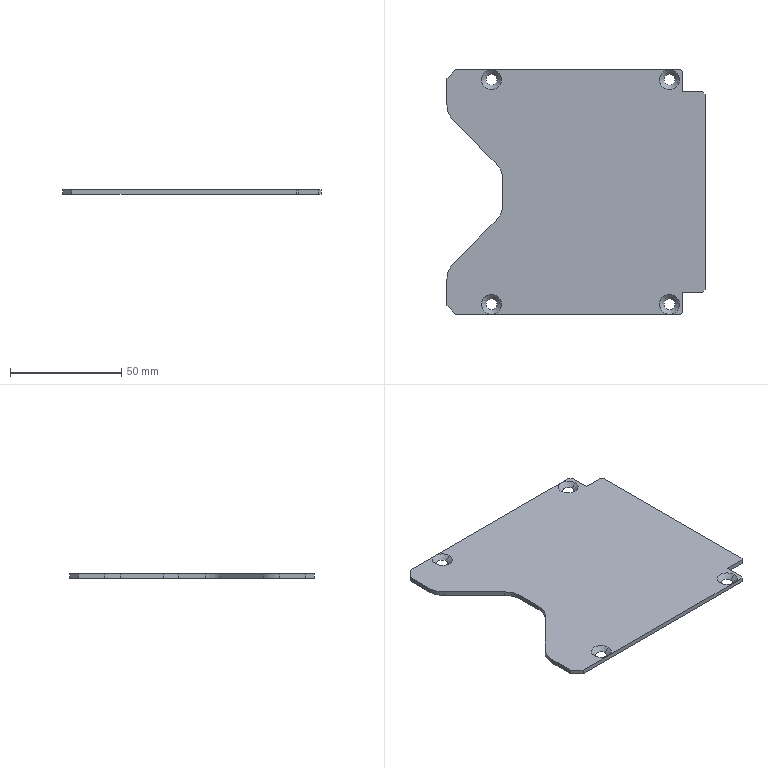Part | SolidWorks | features Chamfer 2, ICE 2, Fillet 1, FlatPattern 1, HoleWzd 1, SMBaseFlange 1, SheetMetal 1 | 1 solid | 32 faces | box 116 x 110 x 2 mm | volume 22518 mm3 | plane 20 | cone 8 | cylinder 4 | commonest cylinder face diameters 20 x4
STEP:
#1=CARTESIAN_POINT('',(-40.5,50.5,-2.));
#2=VERTEX_POINT('',#1);
#3=CARTESIAN_POINT('',(-35.5,50.5,-2.));
#4=VERTEX_POINT('',#3);
#5=CARTESIAN_POINT('',(-38.,50.5,-2.));
#6=DIRECTION('',(0.,0.,1.));
#7=DIRECTION('',(1.,0.,0.));
#8=AXIS2_PLACEMENT_3D('',#5,#6,#7);
#9=CIRCLE('',#8,2.5);
#10=EDGE_CURVE('',#2,#4,#9,.T.);
#11=ORIENTED_EDGE('',*,*,#10,.F.);
#12=CARTESIAN_POINT('',(-42.5,50.5,0.));
#13=VERTEX_POINT('',#12);
#14=CARTESIAN_POINT('',(-42.5,50.5,0.));
#15=DIRECTION('',(-0.7071,0.,0.7071));
#16=VECTOR('',#15,1000.);
#17=LINE('',#14,#16);
#18=EDGE_CURVE('',#2,#13,#17,.T.);
#19=ORIENTED_EDGE('',*,*,#18,.T.);
#20=CARTESIAN_POINT('',(-33.5,50.5,0.));
#21=VERTEX_POINT('',#20);
#22=CARTESIAN_POINT('',(-38.,50.5,0.));
#23=DIRECTION('',(0.,0.,1.));
#24=DIRECTION('',(1.,0.,0.));
#25=AXIS2_PLACEMENT_3D('',#22,#23,#24);
#26=CIRCLE('',#25,4.5);
#27=EDGE_CURVE('',#13,#21,#26,.T.);
#28=ORIENTED_EDGE('',*,*,#27,.T.);
#29=CARTESIAN_POINT('',(-33.5,50.5,0.));
#30=DIRECTION('',(0.7071,0.,0.7071));
#31=VECTOR('',#30,1000.);
#32=LINE('',#29,#31);
#33=EDGE_CURVE('',#4,#21,#32,.T.);
#34=ORIENTED_EDGE('',*,*,#33,.F.);
#35=EDGE_LOOP('',(#11,#19,#28,#34));
#36=FACE_OUTER_BOUND('',#35,.T.);
#37=CARTESIAN_POINT('',(-38.,50.5,0.));
#38=DIRECTION('',(0.,0.,1.));
#39=DIRECTION('',(1.,0.,0.));
#40=AXIS2_PLACEMENT_3D('',#37,#38,#39);
#41=CONICAL_SURFACE('',#40,4.5,0.7854);
#42=ADVANCED_FACE('',(#36),#41,.F.);
#43=CARTESIAN_POINT('',(39.5,50.5,-2.));
#44=VERTEX_POINT('',#43);
#45=CARTESIAN_POINT('',(44.5,50.5,-2.));
#46=VERTEX_POINT('',#45);
#47=CARTESIAN_POINT('',(42.,50.5,-2.));
#48=DIRECTION('',(0.,0.,1.));
#49=DIRECTION('',(1.,0.,0.));
#50=AXIS2_PLACEMENT_3D('',#47,#48,#49);
#51=CIRCLE('',#50,2.5);
#52=EDGE_CURVE('',#44,#46,#51,.T.);
#53=ORIENTED_EDGE('',*,*,#52,.F.);
#54=CARTESIAN_POINT('',(37.5,50.5,0.));
#55=VERTEX_POINT('',#54);
#56=CARTESIAN_POINT('',(37.5,50.5,0.));
#57=DIRECTION('',(-0.7071,0.,0.7071));
#58=VECTOR('',#57,1000.);
#59=LINE('',#56,#58);
#60=EDGE_CURVE('',#44,#55,#59,.T.);
#61=ORIENTED_EDGE('',*,*,#60,.T.);
#62=CARTESIAN_POINT('',(46.5,50.5,0.));
#63=VERTEX_POINT('',#62);
#64=CARTESIAN_POINT('',(42.,50.5,0.));
#65=DIRECTION('',(0.,0.,1.));
#66=DIRECTION('',(1.,0.,0.));
#67=AXIS2_PLACEMENT_3D('',#64,#65,#66);
#68=CIRCLE('',#67,4.5);
#69=EDGE_CURVE('',#55,#63,#68,.T.);
#70=ORIENTED_EDGE('',*,*,#69,.T.);
#71=CARTESIAN_POINT('',(46.5,50.5,0.));
#72=DIRECTION('',(0.7071,0.,0.7071));
#73=VECTOR('',#72,1000.);
#74=LINE('',#71,#73);
#75=EDGE_CURVE('',#46,#63,#74,.T.);
#76=ORIENTED_EDGE('',*,*,#75,.F.);
#77=EDGE_LOOP('',(#53,#61,#70,#76));
#78=FACE_OUTER_BOUND('',#77,.T.);
#79=CARTESIAN_POINT('',(42.,50.5,0.));
#80=DIRECTION('',(0.,0.,1.));
#81=DIRECTION('',(1.,0.,0.));
#82=AXIS2_PLACEMENT_3D('',#79,#80,#81);
#83=CONICAL_SURFACE('',#82,4.5,0.7854);
#84=ADVANCED_FACE('',(#78),#83,.F.);
#85=CARTESIAN_POINT('',(-40.5,-50.5,-2.));
#86=VERTEX_POINT('',#85);
#87=CARTESIAN_POINT('',(-35.5,-50.5,-2.));
#88=VERTEX_POINT('',#87);
#89=CARTESIAN_POINT('',(-38.,-50.5,-2.));
#90=DIRECTION('',(0.,0.,1.));
#91=DIRECTION('',(1.,0.,0.));
#92=AXIS2_PLACEMENT_3D('',#89,#90,#91);
#93=CIRCLE('',#92,2.5);
#94=EDGE_CURVE('',#86,#88,#93,.T.);
#95=ORIENTED_EDGE('',*,*,#94,.F.);
#96=CARTESIAN_POINT('',(-42.5,-50.5,0.));
#97=VERTEX_POINT('',#96);
#98=CARTESIAN_POINT('',(-42.5,-50.5,0.));
#99=DIRECTION('',(-0.7071,0.,0.7071));
#100=VECTOR('',#99,1000.);
#101=LINE('',#98,#100);
#102=EDGE_CURVE('',#86,#97,#101,.T.);
#103=ORIENTED_EDGE('',*,*,#102,.T.);
#104=CARTESIAN_POINT('',(-38.,-55.,0.));
#105=VERTEX_POINT('',#104);
#106=CARTESIAN_POINT('',(-38.,-50.5,0.));
#107=DIRECTION('',(0.,0.,1.));
#108=DIRECTION('',(1.,0.,0.));
#109=AXIS2_PLACEMENT_3D('',#106,#107,#108);
#110=CIRCLE('',#109,4.5);
#111=EDGE_CURVE('',#97,#105,#110,.T.);
#112=ORIENTED_EDGE('',*,*,#111,.T.);
#113=CARTESIAN_POINT('',(-33.5,-50.5,0.));
#114=VERTEX_POINT('',#113);
#115=CARTESIAN_POINT('',(-38.,-50.5,0.));
#116=DIRECTION('',(0.,0.,1.));
#117=DIRECTION('',(1.,0.,0.));
#118=AXIS2_PLACEMENT_3D('',#115,#116,#117);
#119=CIRCLE('',#118,4.5);
#120=EDGE_CURVE('',#105,#114,#119,.T.);
#121=ORIENTED_EDGE('',*,*,#120,.T.);
#122=CARTESIAN_POINT('',(-33.5,-50.5,0.));
#123=DIRECTION('',(0.7071,0.,0.7071));
#124=VECTOR('',#123,1000.);
#125=LINE('',#122,#124);
#126=EDGE_CURVE('',#88,#114,#125,.T.);
#127=ORIENTED_EDGE('',*,*,#126,.F.);
#128=EDGE_LOOP('',(#95,#103,#112,#121,#127));
#129=FACE_OUTER_BOUND('',#128,.T.);
#130=CARTESIAN_POINT('',(-38.,-50.5,0.));
#131=DIRECTION('',(0.,0.,1.));
#132=DIRECTION('',(1.,0.,0.));
#133=AXIS2_PLACEMENT_3D('',#130,#131,#132);
#134=CONICAL_SURFACE('',#133,4.5,0.7854);
#135=ADVANCED_FACE('',(#129),#134,.F.);
#136=CARTESIAN_POINT('',(39.5,-50.5,-2.));
#137=VERTEX_POINT('',#136);
#138=CARTESIAN_POINT('',(44.5,-50.5,-2.));
#139=VERTEX_POINT('',#138);
#140=CARTESIAN_POINT('',(42.,-50.5,-2.));
#141=DIRECTION('',(0.,0.,1.));
#142=DIRECTION('',(1.,0.,0.));
#143=AXIS2_PLACEMENT_3D('',#140,#141,#142);
#144=CIRCLE('',#143,2.5);
#145=EDGE_CURVE('',#137,#139,#144,.T.);
#146=ORIENTED_EDGE('',*,*,#145,.F.);
#147=CARTESIAN_POINT('',(37.5,-50.5,0.));
#148=VERTEX_POINT('',#147);
#149=CARTESIAN_POINT('',(37.5,-50.5,0.));
#150=DIRECTION('',(-0.7071,0.,0.7071));
#151=VECTOR('',#150,1000.);
#152=LINE('',#149,#151);
#153=EDGE_CURVE('',#137,#148,#152,.T.);
#154=ORIENTED_EDGE('',*,*,#153,.T.);
#155=CARTESIAN_POINT('',(42.,-55.,0.));
#156=VERTEX_POINT('',#155);
#157=CARTESIAN_POINT('',(42.,-50.5,0.));
#158=DIRECTION('',(0.,0.,1.));
#159=DIRECTION('',(1.,0.,0.));
#160=AXIS2_PLACEMENT_3D('',#157,#158,#159);
#161=CIRCLE('',#160,4.5);
#162=EDGE_CURVE('',#148,#156,#161,.T.);
#163=ORIENTED_EDGE('',*,*,#162,.T.);
#164=CARTESIAN_POINT('',(46.5,-50.5,0.));
#165=VERTEX_POINT('',#164);
#166=CARTESIAN_POINT('',(42.,-50.5,0.));
#167=DIRECTION('',(0.,0.,1.));
#168=DIRECTION('',(1.,0.,0.));
#169=AXIS2_PLACEMENT_3D('',#166,#167,#168);
#170=CIRCLE('',#169,4.5);
#171=EDGE_CURVE('',#156,#165,#170,.T.);
#172=ORIENTED_EDGE('',*,*,#171,.T.);
#173=CARTESIAN_POINT('',(46.5,-50.5,0.));
#174=DIRECTION('',(0.7071,0.,0.7071));
#175=VECTOR('',#174,1000.);
#176=LINE('',#173,#175);
#177=EDGE_CURVE('',#139,#165,#176,.T.);
#178=ORIENTED_EDGE('',*,*,#177,.F.);
#179=EDGE_LOOP('',(#146,#154,#163,#172,#178));
#180=FACE_OUTER_BOUND('',#179,.T.);
#181=CARTESIAN_POINT('',(42.,-50.5,0.));
#182=DIRECTION('',(0.,0.,1.));
#183=DIRECTION('',(1.,0.,0.));
#184=AXIS2_PLACEMENT_3D('',#181,#182,#183);
#185=CONICAL_SURFACE('',#184,4.5,0.7854);
#186=ADVANCED_FACE('',(#180),#185,.F.);
#187=CARTESIAN_POINT('',(-38.,50.5,-2.));
#188=DIRECTION('',(0.,0.,1.));
#189=DIRECTION('',(1.,0.,0.));
#190=AXIS2_PLACEMENT_3D('',#187,#188,#189);
#191=CIRCLE('',#190,2.5);
#192=EDGE_CURVE('',#4,#2,#191,.T.);
#193=ORIENTED_EDGE('',*,*,#192,.T.);
#194=ORIENTED_EDGE('',*,*,#10,.T.);
#195=EDGE_LOOP('',(#193,#194));
#196=FACE_BOUND('',#195,.T.);
#197=CARTESIAN_POINT('',(-38.,-50.5,-2.));
#198=DIRECTION('',(0.,0.,1.));
#199=DIRECTION('',(1.,0.,0.));
#200=AXIS2_PLACEMENT_3D('',#197,#198,#199);
#201=CIRCLE('',#200,2.5);
#202=EDGE_CURVE('',#88,#86,#201,.T.);
#203=ORIENTED_EDGE('',*,*,#202,.T.);
#204=ORIENTED_EDGE('',*,*,#94,.T.);
#205=EDGE_LOOP('',(#203,#204));
#206=FACE_BOUND('',#205,.T.);
#207=CARTESIAN_POINT('',(-54.,-55.,-2.));
#208=VERTEX_POINT('',#207);
#209=CARTESIAN_POINT('',(47.,-55.,-2.));
#210=VERTEX_POINT('',#209);
#211=CARTESIAN_POINT('',(-58.,-55.,-2.));
#212=DIRECTION('',(1.,0.,0.));
#213=VECTOR('',#212,1000.);
#214=LINE('',#211,#213);
#215=EDGE_CURVE('',#208,#210,#214,.T.);
#216=ORIENTED_EDGE('',*,*,#215,.F.);
#217=CARTESIAN_POINT('',(-58.,-51.,-2.));
#218=VERTEX_POINT('',#217);
#219=CARTESIAN_POINT('',(-58.,-51.,-2.));
#220=DIRECTION('',(-0.7071,0.7071,0.));
#221=VECTOR('',#220,1000.);
#222=LINE('',#219,#221);
#223=EDGE_CURVE('',#208,#218,#222,.T.);
#224=ORIENTED_EDGE('',*,*,#223,.T.);
#225=CARTESIAN_POINT('',(-58.,-39.142,-2.));
#226=VERTEX_POINT('',#225);
#227=CARTESIAN_POINT('',(-58.,55.,-2.));
#228=DIRECTION('',(0.,-1.,0.));
#229=VECTOR('',#228,1000.);
#230=LINE('',#227,#229);
#231=EDGE_CURVE('',#226,#218,#230,.T.);
#232=ORIENTED_EDGE('',*,*,#231,.F.);
#233=CARTESIAN_POINT('',(-55.071,-32.071,-2.));
#234=VERTEX_POINT('',#233);
#235=CARTESIAN_POINT('',(-48.,-39.142,-2.));
#236=DIRECTION('',(0.,0.,-1.));
#237=DIRECTION('',(1.,0.,0.));
#238=AXIS2_PLACEMENT_3D('',#235,#236,#237);
#239=CIRCLE('',#238,10.);
#240=EDGE_CURVE('',#226,#234,#239,.T.);
#241=ORIENTED_EDGE('',*,*,#240,.T.);
#242=CARTESIAN_POINT('',(-35.929,-12.929,-2.));
#243=VERTEX_POINT('',#242);
#244=CARTESIAN_POINT('',(-33.,-10.,-2.));
#245=DIRECTION('',(0.7071,0.7071,0.));
#246=VECTOR('',#245,1000.);
#247=LINE('',#244,#246);
#248=EDGE_CURVE('',#234,#243,#247,.T.);
#249=ORIENTED_EDGE('',*,*,#248,.T.);
#250=CARTESIAN_POINT('',(-33.,-5.858,-2.));
#251=VERTEX_POINT('',#250);
#252=CARTESIAN_POINT('',(-43.,-5.858,-2.));
#253=DIRECTION('',(0.,0.,1.));
#254=DIRECTION('',(1.,0.,0.));
#255=AXIS2_PLACEMENT_3D('',#252,#253,#254);
#256=CIRCLE('',#255,10.);
#257=EDGE_CURVE('',#243,#251,#256,.T.);
#258=ORIENTED_EDGE('',*,*,#257,.T.);
#259=CARTESIAN_POINT('',(-33.,5.858,-2.));
#260=VERTEX_POINT('',#259);
#261=CARTESIAN_POINT('',(-33.,0.,-2.));
#262=DIRECTION('',(0.,1.,0.));
#263=VECTOR('',#262,1000.);
#264=LINE('',#261,#263);
#265=EDGE_CURVE('',#251,#260,#264,.T.);
#266=ORIENTED_EDGE('',*,*,#265,.T.);
#267=CARTESIAN_POINT('',(-35.929,12.929,-2.));
#268=VERTEX_POINT('',#267);
#269=CARTESIAN_POINT('',(-43.,5.858,-2.));
#270=DIRECTION('',(0.,0.,1.));
#271=DIRECTION('',(1.,0.,0.));
#272=AXIS2_PLACEMENT_3D('',#269,#270,#271);
#273=CIRCLE('',#272,10.);
#274=EDGE_CURVE('',#260,#268,#273,.T.);
#275=ORIENTED_EDGE('',*,*,#274,.T.);
#276=CARTESIAN_POINT('',(-55.071,32.071,-2.));
#277=VERTEX_POINT('',#276);
#278=CARTESIAN_POINT('',(-58.,35.,-2.));
#279=DIRECTION('',(-0.7071,0.7071,0.));
#280=VECTOR('',#279,1000.);
#281=LINE('',#278,#280);
#282=EDGE_CURVE('',#268,#277,#281,.T.);
#283=ORIENTED_EDGE('',*,*,#282,.T.);
#284=CARTESIAN_POINT('',(-58.,39.142,-2.));
#285=VERTEX_POINT('',#284);
#286=CARTESIAN_POINT('',(-48.,39.142,-2.));
#287=DIRECTION('',(0.,0.,-1.));
#288=DIRECTION('',(1.,0.,0.));
#289=AXIS2_PLACEMENT_3D('',#286,#287,#288);
#290=CIRCLE('',#289,10.);
#291=EDGE_CURVE('',#277,#285,#290,.T.);
#292=ORIENTED_EDGE('',*,*,#291,.T.);
#293=CARTESIAN_POINT('',(-58.,51.,-2.));
#294=VERTEX_POINT('',#293);
#295=CARTESIAN_POINT('',(-58.,55.,-2.));
#296=DIRECTION('',(0.,-1.,0.));
#297=VECTOR('',#296,1000.);
#298=LINE('',#295,#297);
#299=EDGE_CURVE('',#294,#285,#298,.T.);
#300=ORIENTED_EDGE('',*,*,#299,.F.);
#301=CARTESIAN_POINT('',(-54.,55.,-2.));
#302=VERTEX_POINT('',#301);
#303=CARTESIAN_POINT('',(-54.,55.,-2.));
#304=DIRECTION('',(0.7071,0.7071,0.));
#305=VECTOR('',#304,1000.);
#306=LINE('',#303,#305);
#307=EDGE_CURVE('',#294,#302,#306,.T.);
#308=ORIENTED_EDGE('',*,*,#307,.T.);
#309=CARTESIAN_POINT('',(47.,55.,-2.));
#310=VERTEX_POINT('',#309);
#311=CARTESIAN_POINT('',(-58.,55.,-2.));
#312=DIRECTION('',(-1.,0.,0.));
#313=VECTOR('',#312,1000.);
#314=LINE('',#311,#313);
#315=EDGE_CURVE('',#310,#302,#314,.T.);
#316=ORIENTED_EDGE('',*,*,#315,.F.);
#317=CARTESIAN_POINT('',(48.,54.,-2.));
#318=VERTEX_POINT('',#317);
#319=CARTESIAN_POINT('',(48.,54.,-2.));
#320=DIRECTION('',(0.7071,-0.7071,0.));
#321=VECTOR('',#320,1000.);
#322=LINE('',#319,#321);
#323=EDGE_CURVE('',#310,#318,#322,.T.);
#324=ORIENTED_EDGE('',*,*,#323,.T.);
#325=CARTESIAN_POINT('',(48.,45.,-2.));
#326=VERTEX_POINT('',#325);
#327=CARTESIAN_POINT('',(48.,55.,-2.));
#328=DIRECTION('',(0.,-1.,0.));
#329=VECTOR('',#328,1000.);
#330=LINE('',#327,#329);
#331=EDGE_CURVE('',#318,#326,#330,.T.);
#332=ORIENTED_EDGE('',*,*,#331,.T.);
#333=CARTESIAN_POINT('',(57.,45.,-2.));
#334=VERTEX_POINT('',#333);
#335=CARTESIAN_POINT('',(58.,45.,-2.));
#336=DIRECTION('',(1.,0.,0.));
#337=VECTOR('',#336,1000.);
#338=LINE('',#335,#337);
#339=EDGE_CURVE('',#326,#334,#338,.T.);
#340=ORIENTED_EDGE('',*,*,#339,.T.);
#341=CARTESIAN_POINT('',(58.,44.,-2.));
#342=VERTEX_POINT('',#341);
#343=CARTESIAN_POINT('',(58.,44.,-2.));
#344=DIRECTION('',(0.7071,-0.7071,0.));
#345=VECTOR('',#344,1000.);
#346=LINE('',#343,#345);
#347=EDGE_CURVE('',#334,#342,#346,.T.);
#348=ORIENTED_EDGE('',*,*,#347,.T.);
#349=CARTESIAN_POINT('',(58.,-44.,-2.));
#350=VERTEX_POINT('',#349);
#351=CARTESIAN_POINT('',(58.,55.,-2.));
#352=DIRECTION('',(0.,1.,0.));
#353=VECTOR('',#352,1000.);
#354=LINE('',#351,#353);
#355=EDGE_CURVE('',#350,#342,#354,.T.);
#356=ORIENTED_EDGE('',*,*,#355,.F.);
#357=CARTESIAN_POINT('',(57.,-45.,-2.));
#358=VERTEX_POINT('',#357);
#359=CARTESIAN_POINT('',(57.,-45.,-2.));
#360=DIRECTION('',(-0.7071,-0.7071,0.));
#361=VECTOR('',#360,1000.);
#362=LINE('',#359,#361);
#363=EDGE_CURVE('',#350,#358,#362,.T.);
#364=ORIENTED_EDGE('',*,*,#363,.T.);
#365=CARTESIAN_POINT('',(48.,-45.,-2.));
#366=VERTEX_POINT('',#365);
#367=CARTESIAN_POINT('',(58.,-45.,-2.));
#368=DIRECTION('',(-1.,0.,0.));
#369=VECTOR('',#368,1000.);
#370=LINE('',#367,#369);
#371=EDGE_CURVE('',#358,#366,#370,.T.);
#372=ORIENTED_EDGE('',*,*,#371,.T.);
#373=CARTESIAN_POINT('',(48.,-54.,-2.));
#374=VERTEX_POINT('',#373);
#375=CARTESIAN_POINT('',(48.,-55.,-2.));
#376=DIRECTION('',(0.,-1.,0.));
#377=VECTOR('',#376,1000.);
#378=LINE('',#375,#377);
#379=EDGE_CURVE('',#366,#374,#378,.T.);
#380=ORIENTED_EDGE('',*,*,#379,.T.);
#381=CARTESIAN_POINT('',(47.,-55.,-2.));
#382=DIRECTION('',(-0.7071,-0.7071,0.));
#383=VECTOR('',#382,1000.);
#384=LINE('',#381,#383);
#385=EDGE_CURVE('',#374,#210,#384,.T.);
#386=ORIENTED_EDGE('',*,*,#385,.T.);
#387=EDGE_LOOP('',(#216,#224,#232,#241,#249,#258,#266,#275,#283,#292,#300,#308,#316,#324,#332,#340,#348,#356,#364,#372,#380,#386));
#388=FACE_OUTER_BOUND('',#387,.T.);
#389=CARTESIAN_POINT('',(42.,-50.5,-2.));
#390=DIRECTION('',(0.,0.,1.));
#391=DIRECTION('',(1.,0.,0.));
#392=AXIS2_PLACEMENT_3D('',#389,#390,#391);
#393=CIRCLE('',#392,2.5);
#394=EDGE_CURVE('',#139,#137,#393,.T.);
#395=ORIENTED_EDGE('',*,*,#394,.T.);
#396=ORIENTED_EDGE('',*,*,#145,.T.);
#397=EDGE_LOOP('',(#395,#396));
#398=FACE_BOUND('',#397,.T.);
#399=CARTESIAN_POINT('',(42.,50.5,-2.));
#400=DIRECTION('',(0.,0.,1.));
#401=DIRECTION('',(1.,0.,0.));
#402=AXIS2_PLACEMENT_3D('',#399,#400,#401);
#403=CIRCLE('',#402,2.5);
#404=EDGE_CURVE('',#46,#44,#403,.T.);
#405=ORIENTED_EDGE('',*,*,#404,.T.);
#406=ORIENTED_EDGE('',*,*,#52,.T.);
#407=EDGE_LOOP('',(#405,#406));
#408=FACE_BOUND('',#407,.T.);
#409=CARTESIAN_POINT('',(0.,0.,-2.));
#410=DIRECTION('',(0.,0.,1.));
#411=DIRECTION('',(1.,0.,0.));
#412=AXIS2_PLACEMENT_3D('',#409,#410,#411);
#413=PLANE('',#412);
#414=ADVANCED_FACE('',(#196,#206,#388,#398,#408),#413,.F.);
#415=CARTESIAN_POINT('',(-58.,51.,0.));
#416=VERTEX_POINT('',#415);
#417=CARTESIAN_POINT('',(-58.,39.142,0.));
#418=VERTEX_POINT('',#417);
#419=CARTESIAN_POINT('',(-58.,55.,0.));
#420=DIRECTION('',(0.,-1.,0.));
#421=VECTOR('',#420,1000.);
#422=LINE('',#419,#421);
#423=EDGE_CURVE('',#416,#418,#422,.T.);
#424=ORIENTED_EDGE('',*,*,#423,.F.);
#425=CARTESIAN_POINT('',(-58.,51.,-2.));
#426=DIRECTION('',(0.,0.,-1.));
#427=VECTOR('',#426,1000.);
#428=LINE('',#425,#427);
#429=EDGE_CURVE('',#416,#294,#428,.T.);
#430=ORIENTED_EDGE('',*,*,#429,.T.);
#431=ORIENTED_EDGE('',*,*,#299,.T.);
#432=CARTESIAN_POINT('',(-58.,39.142,-2.));
#433=DIRECTION('',(0.,0.,1.));
#434=VECTOR('',#433,1000.);
#435=LINE('',#432,#434);
#436=EDGE_CURVE('',#285,#418,#435,.T.);
#437=ORIENTED_EDGE('',*,*,#436,.T.);
#438=EDGE_LOOP('',(#424,#430,#431,#437));
#439=FACE_OUTER_BOUND('',#438,.T.);
#440=CARTESIAN_POINT('',(-58.,55.,-2.));
#441=DIRECTION('',(-1.,0.,0.));
#442=DIRECTION('',(0.,-1.,0.));
#443=AXIS2_PLACEMENT_3D('',#440,#441,#442);
#444=PLANE('',#443);
#445=ADVANCED_FACE('',(#439),#444,.T.);
#446=ORIENTED_EDGE('',*,*,#231,.T.);
#447=CARTESIAN_POINT('',(-58.,-51.,0.));
#448=VERTEX_POINT('',#447);
#449=CARTESIAN_POINT('',(-58.,-51.,-2.));
#450=DIRECTION('',(0.,0.,1.));
#451=VECTOR('',#450,1000.);
#452=LINE('',#449,#451);
#453=EDGE_CURVE('',#218,#448,#452,.T.);
#454=ORIENTED_EDGE('',*,*,#453,.T.);
#455=CARTESIAN_POINT('',(-58.,-39.142,0.));
#456=VERTEX_POINT('',#455);
#457=CARTESIAN_POINT('',(-58.,55.,0.));
#458=DIRECTION('',(0.,-1.,0.));
#459=VECTOR('',#458,1000.);
#460=LINE('',#457,#459);
#461=EDGE_CURVE('',#456,#448,#460,.T.);
#462=ORIENTED_EDGE('',*,*,#461,.F.);
#463=CARTESIAN_POINT('',(-58.,-39.142,-2.));
#464=DIRECTION('',(0.,0.,-1.));
#465=VECTOR('',#464,1000.);
#466=LINE('',#463,#465);
#467=EDGE_CURVE('',#456,#226,#466,.T.);
#468=ORIENTED_EDGE('',*,*,#467,.T.);
#469=EDGE_LOOP('',(#446,#454,#462,#468));
#470=FACE_OUTER_BOUND('',#469,.T.);
#471=CARTESIAN_POINT('',(-58.,55.,-2.));
#472=DIRECTION('',(-1.,0.,0.));
#473=DIRECTION('',(0.,-1.,0.));
#474=AXIS2_PLACEMENT_3D('',#471,#472,#473);
#475=PLANE('',#474);
#476=ADVANCED_FACE('',(#470),#475,.T.);
#477=CARTESIAN_POINT('',(42.,55.,0.));
#478=VERTEX_POINT('',#477);
#479=CARTESIAN_POINT('',(-38.,55.,0.));
#480=VERTEX_POINT('',#479);
#481=CARTESIAN_POINT('',(-58.,55.,0.));
#482=DIRECTION('',(-1.,0.,0.));
#483=VECTOR('',#482,1000.);
#484=LINE('',#481,#483);
#485=EDGE_CURVE('',#478,#480,#484,.T.);
#486=ORIENTED_EDGE('',*,*,#485,.T.);
#487=CARTESIAN_POINT('',(-38.,50.5,0.));
#488=DIRECTION('',(0.,0.,1.));
#489=DIRECTION('',(1.,0.,0.));
#490=AXIS2_PLACEMENT_3D('',#487,#488,#489);
#491=CIRCLE('',#490,4.5);
#492=EDGE_CURVE('',#21,#480,#491,.T.);
#493=ORIENTED_EDGE('',*,*,#492,.F.);
#494=ORIENTED_EDGE('',*,*,#27,.F.);
#495=CARTESIAN_POINT('',(-38.,50.5,0.));
#496=DIRECTION('',(0.,0.,1.));
#497=DIRECTION('',(1.,0.,0.));
#498=AXIS2_PLACEMENT_3D('',#495,#496,#497);
#499=CIRCLE('',#498,4.5);
#500=EDGE_CURVE('',#480,#13,#499,.T.);
#501=ORIENTED_EDGE('',*,*,#500,.F.);
#502=CARTESIAN_POINT('',(-54.,55.,0.));
#503=VERTEX_POINT('',#502);
#504=CARTESIAN_POINT('',(-58.,55.,0.));
#505=DIRECTION('',(-1.,0.,0.));
#506=VECTOR('',#505,1000.);
#507=LINE('',#504,#506);
#508=EDGE_CURVE('',#480,#503,#507,.T.);
#509=ORIENTED_EDGE('',*,*,#508,.T.);
#510=CARTESIAN_POINT('',(-54.5,54.5,0.));
#511=DIRECTION('',(-0.7071,-0.7071,0.));
#512=VECTOR('',#511,1000.);
#513=LINE('',#510,#512);
#514=EDGE_CURVE('',#503,#416,#513,.T.);
#515=ORIENTED_EDGE('',*,*,#514,.T.);
#516=ORIENTED_EDGE('',*,*,#423,.T.);
#517=CARTESIAN_POINT('',(-55.071,32.071,0.));
#518=VERTEX_POINT('',#517);
#519=CARTESIAN_POINT('',(-48.,39.142,0.));
#520=DIRECTION('',(0.,0.,1.));
#521=DIRECTION('',(1.,0.,0.));
#522=AXIS2_PLACEMENT_3D('',#519,#520,#521);
#523=CIRCLE('',#522,10.);
#524=EDGE_CURVE('',#418,#518,#523,.T.);
#525=ORIENTED_EDGE('',*,*,#524,.T.);
#526=CARTESIAN_POINT('',(-35.929,12.929,0.));
#527=VERTEX_POINT('',#526);
#528=CARTESIAN_POINT('',(-58.,35.,0.));
#529=DIRECTION('',(-0.7071,0.7071,0.));
#530=VECTOR('',#529,1000.);
#531=LINE('',#528,#530);
#532=EDGE_CURVE('',#527,#518,#531,.T.);
#533=ORIENTED_EDGE('',*,*,#532,.F.);
#534=CARTESIAN_POINT('',(-33.,5.858,0.));
#535=VERTEX_POINT('',#534);
#536=CARTESIAN_POINT('',(-43.,5.858,0.));
#537=DIRECTION('',(0.,0.,-1.));
#538=DIRECTION('',(1.,0.,0.));
#539=AXIS2_PLACEMENT_3D('',#536,#537,#538);
#540=CIRCLE('',#539,10.);
#541=EDGE_CURVE('',#527,#535,#540,.T.);
#542=ORIENTED_EDGE('',*,*,#541,.T.);
#543=CARTESIAN_POINT('',(-33.,-5.858,0.));
#544=VERTEX_POINT('',#543);
#545=CARTESIAN_POINT('',(-33.,10.,0.));
#546=DIRECTION('',(0.,1.,0.));
#547=VECTOR('',#546,1000.);
#548=LINE('',#545,#547);
#549=EDGE_CURVE('',#544,#535,#548,.T.);
#550=ORIENTED_EDGE('',*,*,#549,.F.);
#551=CARTESIAN_POINT('',(-35.929,-12.929,0.));
#552=VERTEX_POINT('',#551);
#553=CARTESIAN_POINT('',(-43.,-5.858,0.));
#554=DIRECTION('',(0.,0.,-1.));
#555=DIRECTION('',(1.,0.,0.));
#556=AXIS2_PLACEMENT_3D('',#553,#554,#555);
#557=CIRCLE('',#556,10.);
#558=EDGE_CURVE('',#544,#552,#557,.T.);
#559=ORIENTED_EDGE('',*,*,#558,.T.);
#560=CARTESIAN_POINT('',(-55.071,-32.071,0.));
#561=VERTEX_POINT('',#560);
#562=CARTESIAN_POINT('',(-33.,-10.,0.));
#563=DIRECTION('',(0.7071,0.7071,0.));
#564=VECTOR('',#563,1000.);
#565=LINE('',#562,#564);
#566=EDGE_CURVE('',#561,#552,#565,.T.);
#567=ORIENTED_EDGE('',*,*,#566,.F.);
#568=CARTESIAN_POINT('',(-48.,-39.142,0.));
#569=DIRECTION('',(0.,0.,1.));
#570=DIRECTION('',(1.,0.,0.));
#571=AXIS2_PLACEMENT_3D('',#568,#569,#570);
#572=CIRCLE('',#571,10.);
#573=EDGE_CURVE('',#561,#456,#572,.T.);
#574=ORIENTED_EDGE('',*,*,#573,.T.);
#575=ORIENTED_EDGE('',*,*,#461,.T.);
#576=CARTESIAN_POINT('',(-54.,-55.,0.));
#577=VERTEX_POINT('',#576);
#578=CARTESIAN_POINT('',(-54.5,-54.5,0.));
#579=DIRECTION('',(0.7071,-0.7071,0.));
#580=VECTOR('',#579,1000.);
#581=LINE('',#578,#580);
#582=EDGE_CURVE('',#448,#577,#581,.T.);
#583=ORIENTED_EDGE('',*,*,#582,.T.);
#584=CARTESIAN_POINT('',(-58.,-55.,0.));
#585=DIRECTION('',(1.,0.,0.));
#586=VECTOR('',#585,1000.);
#587=LINE('',#584,#586);
#588=EDGE_CURVE('',#577,#105,#587,.T.);
#589=ORIENTED_EDGE('',*,*,#588,.T.);
#590=ORIENTED_EDGE('',*,*,#111,.F.);
#591=CARTESIAN_POINT('',(-38.,-50.5,0.));
#592=DIRECTION('',(0.,0.,1.));
#593=DIRECTION('',(1.,0.,0.));
#594=AXIS2_PLACEMENT_3D('',#591,#592,#593);
#595=CIRCLE('',#594,4.5);
#596=EDGE_CURVE('',#114,#97,#595,.T.);
#597=ORIENTED_EDGE('',*,*,#596,.F.);
#598=ORIENTED_EDGE('',*,*,#120,.F.);
#599=CARTESIAN_POINT('',(-58.,-55.,0.));
#600=DIRECTION('',(1.,0.,0.));
#601=VECTOR('',#600,1000.);
#602=LINE('',#599,#601);
#603=EDGE_CURVE('',#105,#156,#602,.T.);
#604=ORIENTED_EDGE('',*,*,#603,.T.);
#605=ORIENTED_EDGE('',*,*,#162,.F.);
#606=CARTESIAN_POINT('',(42.,-50.5,0.));
#607=DIRECTION('',(0.,0.,1.));
#608=DIRECTION('',(1.,0.,0.));
#609=AXIS2_PLACEMENT_3D('',#606,#607,#608);
#610=CIRCLE('',#609,4.5);
#611=EDGE_CURVE('',#165,#148,#610,.T.);
#612=ORIENTED_EDGE('',*,*,#611,.F.);
#613=ORIENTED_EDGE('',*,*,#171,.F.);
#614=CARTESIAN_POINT('',(47.,-55.,0.));
#615=VERTEX_POINT('',#614);
#616=CARTESIAN_POINT('',(-58.,-55.,0.));
#617=DIRECTION('',(1.,0.,0.));
#618=VECTOR('',#617,1000.);
#619=LINE('',#616,#618);
#620=EDGE_CURVE('',#156,#615,#619,.T.);
#621=ORIENTED_EDGE('',*,*,#620,.T.);
#622=CARTESIAN_POINT('',(48.,-54.,0.));
#623=VERTEX_POINT('',#622);
#624=CARTESIAN_POINT('',(51.,-51.,0.));
#625=DIRECTION('',(0.7071,0.7071,0.));
#626=VECTOR('',#625,1000.);
#627=LINE('',#624,#626);
#628=EDGE_CURVE('',#615,#623,#627,.T.);
#629=ORIENTED_EDGE('',*,*,#628,.T.);
#630=CARTESIAN_POINT('',(48.,-45.,0.));
#631=VERTEX_POINT('',#630);
#632=CARTESIAN_POINT('',(48.,-55.,0.));
#633=DIRECTION('',(0.,-1.,0.));
#634=VECTOR('',#633,1000.);
#635=LINE('',#632,#634);
#636=EDGE_CURVE('',#631,#623,#635,.T.);
#637=ORIENTED_EDGE('',*,*,#636,.F.);
#638=CARTESIAN_POINT('',(57.,-45.,0.));
#639=VERTEX_POINT('',#638);
#640=CARTESIAN_POINT('',(58.,-45.,0.));
#641=DIRECTION('',(-1.,0.,0.));
#642=VECTOR('',#641,1000.);
#643=LINE('',#640,#642);
#644=EDGE_CURVE('',#639,#631,#643,.T.);
#645=ORIENTED_EDGE('',*,*,#644,.F.);
#646=CARTESIAN_POINT('',(58.,-44.,0.));
#647=VERTEX_POINT('',#646);
#648=CARTESIAN_POINT('',(51.,-51.,0.));
#649=DIRECTION('',(0.7071,0.7071,0.));
#650=VECTOR('',#649,1000.);
#651=LINE('',#648,#650);
#652=EDGE_CURVE('',#639,#647,#651,.T.);
#653=ORIENTED_EDGE('',*,*,#652,.T.);
#654=CARTESIAN_POINT('',(58.,44.,0.));
#655=VERTEX_POINT('',#654);
#656=CARTESIAN_POINT('',(58.,55.,0.));
#657=DIRECTION('',(0.,1.,0.));
#658=VECTOR('',#657,1000.);
#659=LINE('',#656,#658);
#660=EDGE_CURVE('',#647,#655,#659,.T.);
#661=ORIENTED_EDGE('',*,*,#660,.T.);
#662=CARTESIAN_POINT('',(57.,45.,0.));
#663=VERTEX_POINT('',#662);
#664=CARTESIAN_POINT('',(51.,51.,0.));
#665=DIRECTION('',(-0.7071,0.7071,0.));
#666=VECTOR('',#665,1000.);
#667=LINE('',#664,#666);
#668=EDGE_CURVE('',#655,#663,#667,.T.);
#669=ORIENTED_EDGE('',*,*,#668,.T.);
#670=CARTESIAN_POINT('',(48.,45.,0.));
#671=VERTEX_POINT('',#670);
#672=CARTESIAN_POINT('',(58.,45.,0.));
#673=DIRECTION('',(1.,0.,0.));
#674=VECTOR('',#673,1000.);
#675=LINE('',#672,#674);
#676=EDGE_CURVE('',#671,#663,#675,.T.);
#677=ORIENTED_EDGE('',*,*,#676,.F.);
#678=CARTESIAN_POINT('',(48.,54.,0.));
#679=VERTEX_POINT('',#678);
#680=CARTESIAN_POINT('',(48.,55.,0.));
#681=DIRECTION('',(0.,-1.,0.));
#682=VECTOR('',#681,1000.);
#683=LINE('',#680,#682);
#684=EDGE_CURVE('',#679,#671,#683,.T.);
#685=ORIENTED_EDGE('',*,*,#684,.F.);
#686=CARTESIAN_POINT('',(47.,55.,0.));
#687=VERTEX_POINT('',#686);
#688=CARTESIAN_POINT('',(51.,51.,0.));
#689=DIRECTION('',(-0.7071,0.7071,0.));
#690=VECTOR('',#689,1000.);
#691=LINE('',#688,#690);
#692=EDGE_CURVE('',#679,#687,#691,.T.);
#693=ORIENTED_EDGE('',*,*,#692,.T.);
#694=CARTESIAN_POINT('',(-58.,55.,0.));
#695=DIRECTION('',(-1.,0.,0.));
#696=VECTOR('',#695,1000.);
#697=LINE('',#694,#696);
#698=EDGE_CURVE('',#687,#478,#697,.T.);
#699=ORIENTED_EDGE('',*,*,#698,.T.);
#700=CARTESIAN_POINT('',(42.,50.5,0.));
#701=DIRECTION('',(0.,0.,1.));
#702=DIRECTION('',(1.,0.,0.));
#703=AXIS2_PLACEMENT_3D('',#700,#701,#702);
#704=CIRCLE('',#703,4.5);
#705=EDGE_CURVE('',#63,#478,#704,.T.);
#706=ORIENTED_EDGE('',*,*,#705,.F.);
#707=ORIENTED_EDGE('',*,*,#69,.F.);
#708=CARTESIAN_POINT('',(42.,50.5,0.));
#709=DIRECTION('',(0.,0.,1.));
#710=DIRECTION('',(1.,0.,0.));
#711=AXIS2_PLACEMENT_3D('',#708,#709,#710);
#712=CIRCLE('',#711,4.5);
#713=EDGE_CURVE('',#478,#55,#712,.T.);
#714=ORIENTED_EDGE('',*,*,#713,.F.);
#715=EDGE_LOOP('',(#486,#493,#494,#501,#509,#515,#516,#525,#533,#542,#550,#559,#567,#574,#575,#583,#589,#590,#597,#598,#604,#605,#612,#613,#621,#629,#637,#645,#653,#661,#669,#677,#685,#693,#699,#706,#707,#714));
#716=FACE_OUTER_BOUND('',#715,.T.);
#717=CARTESIAN_POINT('',(0.,0.,0.));
#718=DIRECTION('',(0.,0.,1.));
#719=DIRECTION('',(1.,0.,0.));
#720=AXIS2_PLACEMENT_3D('',#717,#718,#719);
#721=PLANE('',#720);
#722=ADVANCED_FACE('',(#716),#721,.T.);
#723=ORIENTED_EDGE('',*,*,#660,.F.);
#724=CARTESIAN_POINT('',(58.,-44.,-2.));
#725=DIRECTION('',(0.,0.,-1.));
#726=VECTOR('',#725,1000.);
#727=LINE('',#724,#726);
#728=EDGE_CURVE('',#647,#350,#727,.T.);
#729=ORIENTED_EDGE('',*,*,#728,.T.);
#730=ORIENTED_EDGE('',*,*,#355,.T.);
#731=CARTESIAN_POINT('',(58.,44.,0.));
#732=DIRECTION('',(0.,0.,1.));
#733=VECTOR('',#732,1000.);
#734=LINE('',#731,#733);
#735=EDGE_CURVE('',#342,#655,#734,.T.);
#736=ORIENTED_EDGE('',*,*,#735,.T.);
#737=EDGE_LOOP('',(#723,#729,#730,#736));
#738=FACE_OUTER_BOUND('',#737,.T.);
#739=CARTESIAN_POINT('',(58.,55.,-2.));
#740=DIRECTION('',(1.,0.,0.));
#741=DIRECTION('',(0.,1.,0.));
#742=AXIS2_PLACEMENT_3D('',#739,#740,#741);
#743=PLANE('',#742);
#744=ADVANCED_FACE('',(#738),#743,.T.);
#745=ORIENTED_EDGE('',*,*,#588,.F.);
#746=CARTESIAN_POINT('',(-54.,-55.,-2.));
#747=DIRECTION('',(0.,0.,-1.));
#748=VECTOR('',#747,1000.);
#749=LINE('',#746,#748);
#750=EDGE_CURVE('',#577,#208,#749,.T.);
#751=ORIENTED_EDGE('',*,*,#750,.T.);
#752=ORIENTED_EDGE('',*,*,#215,.T.);
#753=CARTESIAN_POINT('',(47.,-55.,0.));
#754=DIRECTION('',(0.,0.,1.));
#755=VECTOR('',#754,1000.);
#756=LINE('',#753,#755);
#757=EDGE_CURVE('',#210,#615,#756,.T.);
#758=ORIENTED_EDGE('',*,*,#757,.T.);
#759=ORIENTED_EDGE('',*,*,#620,.F.);
#760=ORIENTED_EDGE('',*,*,#603,.F.);
#761=EDGE_LOOP('',(#745,#751,#752,#758,#759,#760));
#762=FACE_OUTER_BOUND('',#761,.T.);
#763=CARTESIAN_POINT('',(-58.,-55.,-2.));
#764=DIRECTION('',(0.,-1.,0.));
#765=DIRECTION('',(0.,0.,-1.));
#766=AXIS2_PLACEMENT_3D('',#763,#764,#765);
#767=PLANE('',#766);
#768=ADVANCED_FACE('',(#762),#767,.T.);
#769=ORIENTED_EDGE('',*,*,#315,.T.);
#770=CARTESIAN_POINT('',(-54.,55.,-2.));
#771=DIRECTION('',(0.,0.,1.));
#772=VECTOR('',#771,1000.);
#773=LINE('',#770,#772);
#774=EDGE_CURVE('',#302,#503,#773,.T.);
#775=ORIENTED_EDGE('',*,*,#774,.T.);
#776=ORIENTED_EDGE('',*,*,#508,.F.);
#777=ORIENTED_EDGE('',*,*,#485,.F.);
#778=ORIENTED_EDGE('',*,*,#698,.F.);
#779=CARTESIAN_POINT('',(47.,55.,-2.));
#780=DIRECTION('',(0.,0.,-1.));
#781=VECTOR('',#780,1000.);
#782=LINE('',#779,#781);
#783=EDGE_CURVE('',#687,#310,#782,.T.);
#784=ORIENTED_EDGE('',*,*,#783,.T.);
#785=EDGE_LOOP('',(#769,#775,#776,#777,#778,#784));
#786=FACE_OUTER_BOUND('',#785,.T.);
#787=CARTESIAN_POINT('',(-58.,55.,-2.));
#788=DIRECTION('',(0.,1.,0.));
#789=DIRECTION('',(0.,0.,1.));
#790=AXIS2_PLACEMENT_3D('',#787,#788,#789);
#791=PLANE('',#790);
#792=ADVANCED_FACE('',(#786),#791,.T.);
#793=ORIENTED_EDGE('',*,*,#265,.F.);
#794=CARTESIAN_POINT('',(-33.,-5.858,0.));
#795=DIRECTION('',(0.,0.,1.));
#796=VECTOR('',#795,1000.);
#797=LINE('',#794,#796);
#798=EDGE_CURVE('',#251,#544,#797,.T.);
#799=ORIENTED_EDGE('',*,*,#798,.T.);
#800=ORIENTED_EDGE('',*,*,#549,.T.);
#801=CARTESIAN_POINT('',(-33.,5.858,-2.));
#802=DIRECTION('',(0.,0.,-1.));
#803=VECTOR('',#802,1000.);
#804=LINE('',#801,#803);
#805=EDGE_CURVE('',#535,#260,#804,.T.);
#806=ORIENTED_EDGE('',*,*,#805,.T.);
#807=EDGE_LOOP('',(#793,#799,#800,#806));
#808=FACE_OUTER_BOUND('',#807,.T.);
#809=CARTESIAN_POINT('',(-33.,10.,0.));
#810=DIRECTION('',(1.,0.,0.));
#811=DIRECTION('',(0.,1.,0.));
#812=AXIS2_PLACEMENT_3D('',#809,#810,#811);
#813=PLANE('',#812);
#814=ADVANCED_FACE('',(#808),#813,.F.);
#815=ORIENTED_EDGE('',*,*,#282,.F.);
#816=CARTESIAN_POINT('',(-35.929,12.929,0.));
#817=DIRECTION('',(0.,0.,1.));
#818=VECTOR('',#817,1000.);
#819=LINE('',#816,#818);
#820=EDGE_CURVE('',#268,#527,#819,.T.);
#821=ORIENTED_EDGE('',*,*,#820,.T.);
#822=ORIENTED_EDGE('',*,*,#532,.T.);
#823=CARTESIAN_POINT('',(-55.071,32.071,0.));
#824=DIRECTION('',(0.,0.,-1.));
#825=VECTOR('',#824,1000.);
#826=LINE('',#823,#825);
#827=EDGE_CURVE('',#518,#277,#826,.T.);
#828=ORIENTED_EDGE('',*,*,#827,.T.);
#829=EDGE_LOOP('',(#815,#821,#822,#828));
#830=FACE_OUTER_BOUND('',#829,.T.);
#831=CARTESIAN_POINT('',(-58.,35.,0.));
#832=DIRECTION('',(0.7071,0.7071,0.));
#833=DIRECTION('',(-0.7071,0.7071,0.));
#834=AXIS2_PLACEMENT_3D('',#831,#832,#833);
#835=PLANE('',#834);
#836=ADVANCED_FACE('',(#830),#835,.F.);
#837=ORIENTED_EDGE('',*,*,#248,.F.);
#838=CARTESIAN_POINT('',(-55.071,-32.071,0.));
#839=DIRECTION('',(0.,0.,1.));
#840=VECTOR('',#839,1000.);
#841=LINE('',#838,#840);
#842=EDGE_CURVE('',#234,#561,#841,.T.);
#843=ORIENTED_EDGE('',*,*,#842,.T.);
#844=ORIENTED_EDGE('',*,*,#566,.T.);
#845=CARTESIAN_POINT('',(-35.929,-12.929,-2.));
#846=DIRECTION('',(0.,0.,-1.));
#847=VECTOR('',#846,1000.);
#848=LINE('',#845,#847);
#849=EDGE_CURVE('',#552,#243,#848,.T.);
#850=ORIENTED_EDGE('',*,*,#849,.T.);
#851=EDGE_LOOP('',(#837,#843,#844,#850));
#852=FACE_OUTER_BOUND('',#851,.T.);
#853=CARTESIAN_POINT('',(-33.,-10.,0.));
#854=DIRECTION('',(0.7071,-0.7071,0.));
#855=DIRECTION('',(0.7071,0.7071,0.));
#856=AXIS2_PLACEMENT_3D('',#853,#854,#855);
#857=PLANE('',#856);
#858=ADVANCED_FACE('',(#852),#857,.F.);
#859=ORIENTED_EDGE('',*,*,#573,.F.);
#860=ORIENTED_EDGE('',*,*,#842,.F.);
#861=ORIENTED_EDGE('',*,*,#240,.F.);
#862=ORIENTED_EDGE('',*,*,#467,.F.);
#863=EDGE_LOOP('',(#859,#860,#861,#862));
#864=FACE_OUTER_BOUND('',#863,.T.);
#865=CARTESIAN_POINT('',(-48.,-39.142,-2.));
#866=DIRECTION('',(0.,0.,1.));
#867=DIRECTION('',(1.,0.,0.));
#868=AXIS2_PLACEMENT_3D('',#865,#866,#867);
#869=CYLINDRICAL_SURFACE('',#868,10.);
#870=ADVANCED_FACE('',(#864),#869,.T.);
#871=ORIENTED_EDGE('',*,*,#558,.F.);
#872=ORIENTED_EDGE('',*,*,#798,.F.);
#873=ORIENTED_EDGE('',*,*,#257,.F.);
#874=ORIENTED_EDGE('',*,*,#849,.F.);
#875=EDGE_LOOP('',(#871,#872,#873,#874));
#876=FACE_OUTER_BOUND('',#875,.T.);
#877=CARTESIAN_POINT('',(-43.,-5.858,0.));
#878=DIRECTION('',(0.,0.,1.));
#879=DIRECTION('',(1.,0.,0.));
#880=AXIS2_PLACEMENT_3D('',#877,#878,#879);
#881=CYLINDRICAL_SURFACE('',#880,10.);
#882=ADVANCED_FACE('',(#876),#881,.F.);
#883=ORIENTED_EDGE('',*,*,#541,.F.);
#884=ORIENTED_EDGE('',*,*,#820,.F.);
#885=ORIENTED_EDGE('',*,*,#274,.F.);
#886=ORIENTED_EDGE('',*,*,#805,.F.);
#887=EDGE_LOOP('',(#883,#884,#885,#886));
#888=FACE_OUTER_BOUND('',#887,.T.);
#889=CARTESIAN_POINT('',(-43.,5.858,0.));
#890=DIRECTION('',(0.,0.,1.));
#891=DIRECTION('',(1.,0.,0.));
#892=AXIS2_PLACEMENT_3D('',#889,#890,#891);
#893=CYLINDRICAL_SURFACE('',#892,10.);
#894=ADVANCED_FACE('',(#888),#893,.F.);
#895=ORIENTED_EDGE('',*,*,#524,.F.);
#896=ORIENTED_EDGE('',*,*,#436,.F.);
#897=ORIENTED_EDGE('',*,*,#291,.F.);
#898=ORIENTED_EDGE('',*,*,#827,.F.);
#899=EDGE_LOOP('',(#895,#896,#897,#898));
#900=FACE_OUTER_BOUND('',#899,.T.);
#901=CARTESIAN_POINT('',(-48.,39.142,0.));
#902=DIRECTION('',(0.,0.,1.));
#903=DIRECTION('',(1.,0.,0.));
#904=AXIS2_PLACEMENT_3D('',#901,#902,#903);
#905=CYLINDRICAL_SURFACE('',#904,10.);
#906=ADVANCED_FACE('',(#900),#905,.T.);
#907=ORIENTED_EDGE('',*,*,#676,.T.);
#908=CARTESIAN_POINT('',(57.,45.,-2.));
#909=DIRECTION('',(0.,0.,-1.));
#910=VECTOR('',#909,1000.);
#911=LINE('',#908,#910);
#912=EDGE_CURVE('',#663,#334,#911,.T.);
#913=ORIENTED_EDGE('',*,*,#912,.T.);
#914=ORIENTED_EDGE('',*,*,#339,.F.);
#915=CARTESIAN_POINT('',(48.,45.,-2.));
#916=DIRECTION('',(0.,0.,1.));
#917=VECTOR('',#916,1000.);
#918=LINE('',#915,#917);
#919=EDGE_CURVE('',#326,#671,#918,.T.);
#920=ORIENTED_EDGE('',*,*,#919,.T.);
#921=EDGE_LOOP('',(#907,#913,#914,#920));
#922=FACE_OUTER_BOUND('',#921,.T.);
#923=CARTESIAN_POINT('',(58.,45.,-2.));
#924=DIRECTION('',(0.,-1.,0.));
#925=DIRECTION('',(0.,0.,-1.));
#926=AXIS2_PLACEMENT_3D('',#923,#924,#925);
#927=PLANE('',#926);
#928=ADVANCED_FACE('',(#922),#927,.F.);
#929=ORIENTED_EDGE('',*,*,#331,.F.);
#930=CARTESIAN_POINT('',(48.,54.,0.));
#931=DIRECTION('',(0.,0.,1.));
#932=VECTOR('',#931,1000.);
#933=LINE('',#930,#932);
#934=EDGE_CURVE('',#318,#679,#933,.T.);
#935=ORIENTED_EDGE('',*,*,#934,.T.);
#936=ORIENTED_EDGE('',*,*,#684,.T.);
#937=ORIENTED_EDGE('',*,*,#919,.F.);
#938=EDGE_LOOP('',(#929,#935,#936,#937));
#939=FACE_OUTER_BOUND('',#938,.T.);
#940=CARTESIAN_POINT('',(48.,55.,-2.));
#941=DIRECTION('',(-1.,0.,0.));
#942=DIRECTION('',(0.,0.,1.));
#943=AXIS2_PLACEMENT_3D('',#940,#941,#942);
#944=PLANE('',#943);
#945=ADVANCED_FACE('',(#939),#944,.F.);
#946=ORIENTED_EDGE('',*,*,#636,.T.);
#947=CARTESIAN_POINT('',(48.,-54.,-2.));
#948=DIRECTION('',(0.,0.,-1.));
#949=VECTOR('',#948,1000.);
#950=LINE('',#947,#949);
#951=EDGE_CURVE('',#623,#374,#950,.T.);
#952=ORIENTED_EDGE('',*,*,#951,.T.);
#953=ORIENTED_EDGE('',*,*,#379,.F.);
#954=CARTESIAN_POINT('',(48.,-45.,-2.));
#955=DIRECTION('',(0.,0.,1.));
#956=VECTOR('',#955,1000.);
#957=LINE('',#954,#956);
#958=EDGE_CURVE('',#366,#631,#957,.T.);
#959=ORIENTED_EDGE('',*,*,#958,.T.);
#960=EDGE_LOOP('',(#946,#952,#953,#959));
#961=FACE_OUTER_BOUND('',#960,.T.);
#962=CARTESIAN_POINT('',(48.,-55.,-2.));
#963=DIRECTION('',(-1.,0.,0.));
#964=DIRECTION('',(0.,0.,1.));
#965=AXIS2_PLACEMENT_3D('',#962,#963,#964);
#966=PLANE('',#965);
#967=ADVANCED_FACE('',(#961),#966,.F.);
#968=ORIENTED_EDGE('',*,*,#371,.F.);
#969=CARTESIAN_POINT('',(57.,-45.,0.));
#970=DIRECTION('',(0.,0.,1.));
#971=VECTOR('',#970,1000.);
#972=LINE('',#969,#971);
#973=EDGE_CURVE('',#358,#639,#972,.T.);
#974=ORIENTED_EDGE('',*,*,#973,.T.);
#975=ORIENTED_EDGE('',*,*,#644,.T.);
#976=ORIENTED_EDGE('',*,*,#958,.F.);
#977=EDGE_LOOP('',(#968,#974,#975,#976));
#978=FACE_OUTER_BOUND('',#977,.T.);
#979=CARTESIAN_POINT('',(58.,-45.,-2.));
#980=DIRECTION('',(0.,1.,0.));
#981=DIRECTION('',(0.,0.,1.));
#982=AXIS2_PLACEMENT_3D('',#979,#980,#981);
#983=PLANE('',#982);
#984=ADVANCED_FACE('',(#978),#983,.F.);
#985=ORIENTED_EDGE('',*,*,#363,.F.);
#986=ORIENTED_EDGE('',*,*,#728,.F.);
#987=ORIENTED_EDGE('',*,*,#652,.F.);
#988=ORIENTED_EDGE('',*,*,#973,.F.);
#989=EDGE_LOOP('',(#985,#986,#987,#988));
#990=FACE_OUTER_BOUND('',#989,.T.);
#991=CARTESIAN_POINT('',(57.,-45.,-2.));
#992=DIRECTION('',(0.7071,-0.7071,0.));
#993=DIRECTION('',(0.,0.,-1.));
#994=AXIS2_PLACEMENT_3D('',#991,#992,#993);
#995=PLANE('',#994);
#996=ADVANCED_FACE('',(#990),#995,.T.);
#997=ORIENTED_EDGE('',*,*,#385,.F.);
#998=ORIENTED_EDGE('',*,*,#951,.F.);
#999=ORIENTED_EDGE('',*,*,#628,.F.);
#1000=ORIENTED_EDGE('',*,*,#757,.F.);
#1001=EDGE_LOOP('',(#997,#998,#999,#1000));
#1002=FACE_OUTER_BOUND('',#1001,.T.);
#1003=CARTESIAN_POINT('',(47.,-55.,-2.));
#1004=DIRECTION('',(0.7071,-0.7071,0.));
#1005=DIRECTION('',(0.,0.,-1.));
#1006=AXIS2_PLACEMENT_3D('',#1003,#1004,#1005);
#1007=PLANE('',#1006);
#1008=ADVANCED_FACE('',(#1002),#1007,.T.);
#1009=ORIENTED_EDGE('',*,*,#323,.F.);
#1010=ORIENTED_EDGE('',*,*,#783,.F.);
#1011=ORIENTED_EDGE('',*,*,#692,.F.);
#1012=ORIENTED_EDGE('',*,*,#934,.F.);
#1013=EDGE_LOOP('',(#1009,#1010,#1011,#1012));
#1014=FACE_OUTER_BOUND('',#1013,.T.);
#1015=CARTESIAN_POINT('',(48.,54.,-2.));
#1016=DIRECTION('',(0.7071,0.7071,0.));
#1017=DIRECTION('',(0.,0.,-1.));
#1018=AXIS2_PLACEMENT_3D('',#1015,#1016,#1017);
#1019=PLANE('',#1018);
#1020=ADVANCED_FACE('',(#1014),#1019,.T.);
#1021=ORIENTED_EDGE('',*,*,#347,.F.);
#1022=ORIENTED_EDGE('',*,*,#912,.F.);
#1023=ORIENTED_EDGE('',*,*,#668,.F.);
#1024=ORIENTED_EDGE('',*,*,#735,.F.);
#1025=EDGE_LOOP('',(#1021,#1022,#1023,#1024));
#1026=FACE_OUTER_BOUND('',#1025,.T.);
#1027=CARTESIAN_POINT('',(58.,44.,-2.));
#1028=DIRECTION('',(0.7071,0.7071,0.));
#1029=DIRECTION('',(0.,0.,-1.));
#1030=AXIS2_PLACEMENT_3D('',#1027,#1028,#1029);
#1031=PLANE('',#1030);
#1032=ADVANCED_FACE('',(#1026),#1031,.T.);
#1033=ORIENTED_EDGE('',*,*,#223,.F.);
#1034=ORIENTED_EDGE('',*,*,#750,.F.);
#1035=ORIENTED_EDGE('',*,*,#582,.F.);
#1036=ORIENTED_EDGE('',*,*,#453,.F.);
#1037=EDGE_LOOP('',(#1033,#1034,#1035,#1036));
#1038=FACE_OUTER_BOUND('',#1037,.T.);
#1039=CARTESIAN_POINT('',(-58.,-51.,-2.));
#1040=DIRECTION('',(0.7071,0.7071,0.));
#1041=DIRECTION('',(0.,0.,1.));
#1042=AXIS2_PLACEMENT_3D('',#1039,#1040,#1041);
#1043=PLANE('',#1042);
#1044=ADVANCED_FACE('',(#1038),#1043,.F.);
#1045=ORIENTED_EDGE('',*,*,#307,.F.);
#1046=ORIENTED_EDGE('',*,*,#429,.F.);
#1047=ORIENTED_EDGE('',*,*,#514,.F.);
#1048=ORIENTED_EDGE('',*,*,#774,.F.);
#1049=EDGE_LOOP('',(#1045,#1046,#1047,#1048));
#1050=FACE_OUTER_BOUND('',#1049,.T.);
#1051=CARTESIAN_POINT('',(-54.,55.,-2.));
#1052=DIRECTION('',(0.7071,-0.7071,0.));
#1053=DIRECTION('',(0.,0.,1.));
#1054=AXIS2_PLACEMENT_3D('',#1051,#1052,#1053);
#1055=PLANE('',#1054);
#1056=ADVANCED_FACE('',(#1050),#1055,.F.);
#1057=ORIENTED_EDGE('',*,*,#153,.F.);
#1058=ORIENTED_EDGE('',*,*,#394,.F.);
#1059=ORIENTED_EDGE('',*,*,#177,.T.);
#1060=ORIENTED_EDGE('',*,*,#611,.T.);
#1061=EDGE_LOOP('',(#1057,#1058,#1059,#1060));
#1062=FACE_OUTER_BOUND('',#1061,.T.);
#1063=CARTESIAN_POINT('',(42.,-50.5,0.));
#1064=DIRECTION('',(0.,0.,1.));
#1065=DIRECTION('',(1.,0.,0.));
#1066=AXIS2_PLACEMENT_3D('',#1063,#1064,#1065);
#1067=CONICAL_SURFACE('',#1066,4.5,0.7854);
#1068=ADVANCED_FACE('',(#1062),#1067,.F.);
#1069=ORIENTED_EDGE('',*,*,#102,.F.);
#1070=ORIENTED_EDGE('',*,*,#202,.F.);
#1071=ORIENTED_EDGE('',*,*,#126,.T.);
#1072=ORIENTED_EDGE('',*,*,#596,.T.);
#1073=EDGE_LOOP('',(#1069,#1070,#1071,#1072));
#1074=FACE_OUTER_BOUND('',#1073,.T.);
#1075=CARTESIAN_POINT('',(-38.,-50.5,0.));
#1076=DIRECTION('',(0.,0.,1.));
#1077=DIRECTION('',(1.,0.,0.));
#1078=AXIS2_PLACEMENT_3D('',#1075,#1076,#1077);
#1079=CONICAL_SURFACE('',#1078,4.5,0.7854);
#1080=ADVANCED_FACE('',(#1074),#1079,.F.);
#1081=ORIENTED_EDGE('',*,*,#60,.F.);
#1082=ORIENTED_EDGE('',*,*,#404,.F.);
#1083=ORIENTED_EDGE('',*,*,#75,.T.);
#1084=ORIENTED_EDGE('',*,*,#705,.T.);
#1085=ORIENTED_EDGE('',*,*,#713,.T.);
#1086=EDGE_LOOP('',(#1081,#1082,#1083,#1084,#1085));
#1087=FACE_OUTER_BOUND('',#1086,.T.);
#1088=CARTESIAN_POINT('',(42.,50.5,0.));
#1089=DIRECTION('',(0.,0.,1.));
#1090=DIRECTION('',(1.,0.,0.));
#1091=AXIS2_PLACEMENT_3D('',#1088,#1089,#1090);
#1092=CONICAL_SURFACE('',#1091,4.5,0.7854);
#1093=ADVANCED_FACE('',(#1087),#1092,.F.);
#1094=ORIENTED_EDGE('',*,*,#18,.F.);
#1095=ORIENTED_EDGE('',*,*,#192,.F.);
#1096=ORIENTED_EDGE('',*,*,#33,.T.);
#1097=ORIENTED_EDGE('',*,*,#492,.T.);
#1098=ORIENTED_EDGE('',*,*,#500,.T.);
#1099=EDGE_LOOP('',(#1094,#1095,#1096,#1097,#1098));
#1100=FACE_OUTER_BOUND('',#1099,.T.);
#1101=CARTESIAN_POINT('',(-38.,50.5,0.));
#1102=DIRECTION('',(0.,0.,1.));
#1103=DIRECTION('',(1.,0.,0.));
#1104=AXIS2_PLACEMENT_3D('',#1101,#1102,#1103);
#1105=CONICAL_SURFACE('',#1104,4.5,0.7854);
#1106=ADVANCED_FACE('',(#1100),#1105,.F.);
#1107=CLOSED_SHELL('',(#42,#84,#135,#186,#414,#445,#476,#722,#744,#768,#792,#814,#836,#858,#870,#882,#894,#906,#928,#945,#967,#984,#996,#1008,#1020,#1032,#1044,#1056,#1068,#1080,#1093,#1106));
#1108=MANIFOLD_SOLID_BREP('',#1107);
#1109=CARTESIAN_POINT('',(0.,0.,0.));
#1110=DIRECTION('',(0.,0.,1.));
#1111=DIRECTION('',(1.,0.,0.));
#1112=AXIS2_PLACEMENT_3D('',#1109,#1110,#1111);
#1113=(LENGTH_UNIT()NAMED_UNIT(*)SI_UNIT(.MILLI.,.METRE.));
#1114=UNCERTAINTY_MEASURE_WITH_UNIT(LENGTH_MEASURE(0.00001),#1113,'','');
#1115=(NAMED_UNIT(*)PLANE_ANGLE_UNIT()SI_UNIT($,.RADIAN.));
#1116=(NAMED_UNIT(*)SI_UNIT($,.STERADIAN.)SOLID_ANGLE_UNIT());
#1117=(GEOMETRIC_REPRESENTATION_CONTEXT(3)GLOBAL_UNCERTAINTY_ASSIGNED_CONTEXT((#1114))GLOBAL_UNIT_ASSIGNED_CONTEXT((#1113,#1115,#1116))REPRESENTATION_CONTEXT('',''));
#1118=ADVANCED_BREP_SHAPE_REPRESENTATION('',(#1108,#1112),#1117);